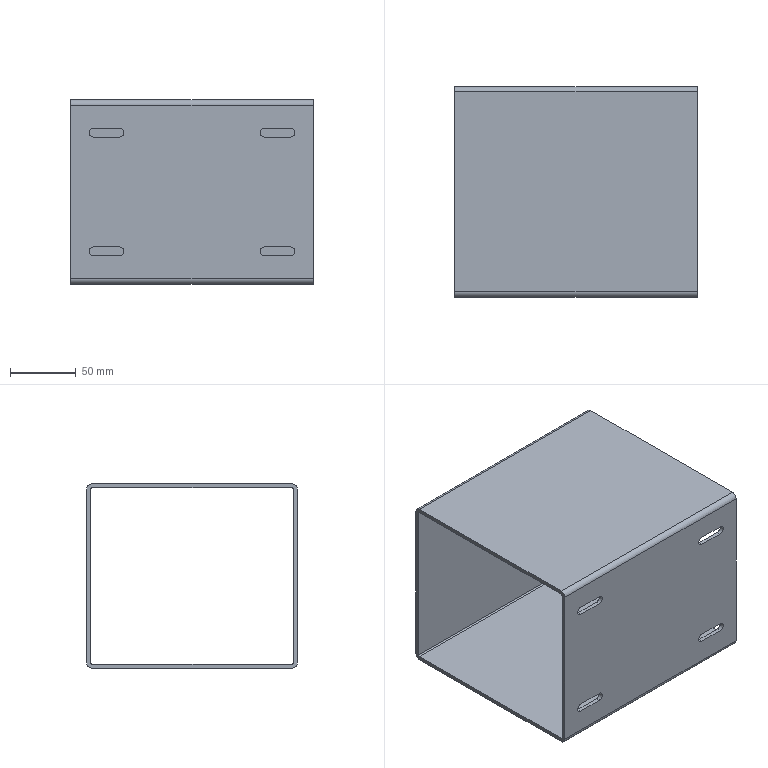Part | SolidWorks | features Fillet 2, Extrusion 1, ICE 1 | 1 solid | 34 faces | box 184 x 160 x 140 mm | volume 320249 mm3 | plane 18 | cylinder 16 | commonest cylinder face diameters 6.5 x8 2 x4 8 x4
STEP:
#1=CARTESIAN_POINT('',(150.,-76.,-70.));
#2=VERTEX_POINT('',#1);
#3=CARTESIAN_POINT('',(150.,76.,-70.));
#4=VERTEX_POINT('',#3);
#5=CARTESIAN_POINT('',(150.,80.,-70.));
#6=DIRECTION('',(0.,1.,0.));
#7=VECTOR('',#6,1000.);
#8=LINE('',#5,#7);
#9=EDGE_CURVE('',#2,#4,#8,.T.);
#10=ORIENTED_EDGE('',*,*,#9,.F.);
#11=CARTESIAN_POINT('',(-34.,-76.,-70.));
#12=VERTEX_POINT('',#11);
#13=CARTESIAN_POINT('',(-34.,-76.,-70.));
#14=DIRECTION('',(-1.,0.,0.));
#15=VECTOR('',#14,1000.);
#16=LINE('',#13,#15);
#17=EDGE_CURVE('',#2,#12,#16,.T.);
#18=ORIENTED_EDGE('',*,*,#17,.T.);
#19=CARTESIAN_POINT('',(-34.,76.,-70.));
#20=VERTEX_POINT('',#19);
#21=CARTESIAN_POINT('',(-34.,80.,-70.));
#22=DIRECTION('',(0.,1.,0.));
#23=VECTOR('',#22,1000.);
#24=LINE('',#21,#23);
#25=EDGE_CURVE('',#12,#20,#24,.T.);
#26=ORIENTED_EDGE('',*,*,#25,.T.);
#27=CARTESIAN_POINT('',(-34.,76.,-70.));
#28=DIRECTION('',(1.,0.,0.));
#29=VECTOR('',#28,1000.);
#30=LINE('',#27,#29);
#31=EDGE_CURVE('',#20,#4,#30,.T.);
#32=ORIENTED_EDGE('',*,*,#31,.T.);
#33=EDGE_LOOP('',(#10,#18,#26,#32));
#34=FACE_OUTER_BOUND('',#33,.T.);
#35=CARTESIAN_POINT('',(-34.,80.,-70.));
#36=DIRECTION('',(0.,0.,-1.));
#37=DIRECTION('',(0.,1.,0.));
#38=AXIS2_PLACEMENT_3D('',#35,#36,#37);
#39=PLANE('',#38);
#40=ADVANCED_FACE('',(#34),#39,.T.);
#41=CARTESIAN_POINT('',(-17.,-80.,48.25));
#42=VERTEX_POINT('',#41);
#43=CARTESIAN_POINT('',(-17.,-80.,41.75));
#44=VERTEX_POINT('',#43);
#45=CARTESIAN_POINT('',(-17.,-80.,45.));
#46=DIRECTION('',(0.,-1.,0.));
#47=DIRECTION('',(0.,0.,-1.));
#48=AXIS2_PLACEMENT_3D('',#45,#46,#47);
#49=CIRCLE('',#48,3.25);
#50=EDGE_CURVE('',#42,#44,#49,.T.);
#51=ORIENTED_EDGE('',*,*,#50,.F.);
#52=CARTESIAN_POINT('',(3.,-80.,48.25));
#53=VERTEX_POINT('',#52);
#54=CARTESIAN_POINT('',(-34.,-80.,48.25));
#55=DIRECTION('',(-1.,0.,0.));
#56=VECTOR('',#55,1000.);
#57=LINE('',#54,#56);
#58=EDGE_CURVE('',#53,#42,#57,.T.);
#59=ORIENTED_EDGE('',*,*,#58,.F.);
#60=CARTESIAN_POINT('',(3.,-80.,41.75));
#61=VERTEX_POINT('',#60);
#62=CARTESIAN_POINT('',(3.,-80.,45.));
#63=DIRECTION('',(0.,-1.,0.));
#64=DIRECTION('',(0.,0.,-1.));
#65=AXIS2_PLACEMENT_3D('',#62,#63,#64);
#66=CIRCLE('',#65,3.25);
#67=EDGE_CURVE('',#61,#53,#66,.T.);
#68=ORIENTED_EDGE('',*,*,#67,.F.);
#69=CARTESIAN_POINT('',(-34.,-80.,41.75));
#70=DIRECTION('',(1.,0.,0.));
#71=VECTOR('',#70,1000.);
#72=LINE('',#69,#71);
#73=EDGE_CURVE('',#44,#61,#72,.T.);
#74=ORIENTED_EDGE('',*,*,#73,.F.);
#75=EDGE_LOOP('',(#51,#59,#68,#74));
#76=FACE_BOUND('',#75,.T.);
#77=CARTESIAN_POINT('',(133.,-80.,-48.25));
#78=VERTEX_POINT('',#77);
#79=CARTESIAN_POINT('',(133.,-80.,-41.75));
#80=VERTEX_POINT('',#79);
#81=CARTESIAN_POINT('',(133.,-80.,-45.));
#82=DIRECTION('',(0.,-1.,0.));
#83=DIRECTION('',(0.,0.,-1.));
#84=AXIS2_PLACEMENT_3D('',#81,#82,#83);
#85=CIRCLE('',#84,3.25);
#86=EDGE_CURVE('',#78,#80,#85,.T.);
#87=ORIENTED_EDGE('',*,*,#86,.F.);
#88=CARTESIAN_POINT('',(113.,-80.,-48.25));
#89=VERTEX_POINT('',#88);
#90=CARTESIAN_POINT('',(-34.,-80.,-48.25));
#91=DIRECTION('',(1.,0.,0.));
#92=VECTOR('',#91,1000.);
#93=LINE('',#90,#92);
#94=EDGE_CURVE('',#89,#78,#93,.T.);
#95=ORIENTED_EDGE('',*,*,#94,.F.);
#96=CARTESIAN_POINT('',(113.,-80.,-41.75));
#97=VERTEX_POINT('',#96);
#98=CARTESIAN_POINT('',(113.,-80.,-45.));
#99=DIRECTION('',(0.,-1.,0.));
#100=DIRECTION('',(0.,0.,-1.));
#101=AXIS2_PLACEMENT_3D('',#98,#99,#100);
#102=CIRCLE('',#101,3.25);
#103=EDGE_CURVE('',#97,#89,#102,.T.);
#104=ORIENTED_EDGE('',*,*,#103,.F.);
#105=CARTESIAN_POINT('',(-34.,-80.,-41.75));
#106=DIRECTION('',(-1.,0.,0.));
#107=VECTOR('',#106,1000.);
#108=LINE('',#105,#107);
#109=EDGE_CURVE('',#80,#97,#108,.T.);
#110=ORIENTED_EDGE('',*,*,#109,.F.);
#111=EDGE_LOOP('',(#87,#95,#104,#110));
#112=FACE_BOUND('',#111,.T.);
#113=CARTESIAN_POINT('',(133.,-80.,41.75));
#114=VERTEX_POINT('',#113);
#115=CARTESIAN_POINT('',(133.,-80.,48.25));
#116=VERTEX_POINT('',#115);
#117=CARTESIAN_POINT('',(133.,-80.,45.));
#118=DIRECTION('',(0.,-1.,0.));
#119=DIRECTION('',(0.,0.,-1.));
#120=AXIS2_PLACEMENT_3D('',#117,#118,#119);
#121=CIRCLE('',#120,3.25);
#122=EDGE_CURVE('',#114,#116,#121,.T.);
#123=ORIENTED_EDGE('',*,*,#122,.F.);
#124=CARTESIAN_POINT('',(113.,-80.,41.75));
#125=VERTEX_POINT('',#124);
#126=CARTESIAN_POINT('',(-34.,-80.,41.75));
#127=DIRECTION('',(1.,0.,0.));
#128=VECTOR('',#127,1000.);
#129=LINE('',#126,#128);
#130=EDGE_CURVE('',#125,#114,#129,.T.);
#131=ORIENTED_EDGE('',*,*,#130,.F.);
#132=CARTESIAN_POINT('',(113.,-80.,48.25));
#133=VERTEX_POINT('',#132);
#134=CARTESIAN_POINT('',(113.,-80.,45.));
#135=DIRECTION('',(0.,-1.,0.));
#136=DIRECTION('',(0.,0.,-1.));
#137=AXIS2_PLACEMENT_3D('',#134,#135,#136);
#138=CIRCLE('',#137,3.25);
#139=EDGE_CURVE('',#133,#125,#138,.T.);
#140=ORIENTED_EDGE('',*,*,#139,.F.);
#141=CARTESIAN_POINT('',(-34.,-80.,48.25));
#142=DIRECTION('',(-1.,0.,0.));
#143=VECTOR('',#142,1000.);
#144=LINE('',#141,#143);
#145=EDGE_CURVE('',#116,#133,#144,.T.);
#146=ORIENTED_EDGE('',*,*,#145,.F.);
#147=EDGE_LOOP('',(#123,#131,#140,#146));
#148=FACE_BOUND('',#147,.T.);
#149=CARTESIAN_POINT('',(-17.,-80.,-41.75));
#150=VERTEX_POINT('',#149);
#151=CARTESIAN_POINT('',(-17.,-80.,-48.25));
#152=VERTEX_POINT('',#151);
#153=CARTESIAN_POINT('',(-17.,-80.,-45.));
#154=DIRECTION('',(0.,-1.,0.));
#155=DIRECTION('',(0.,0.,-1.));
#156=AXIS2_PLACEMENT_3D('',#153,#154,#155);
#157=CIRCLE('',#156,3.25);
#158=EDGE_CURVE('',#150,#152,#157,.T.);
#159=ORIENTED_EDGE('',*,*,#158,.F.);
#160=CARTESIAN_POINT('',(3.,-80.,-41.75));
#161=VERTEX_POINT('',#160);
#162=CARTESIAN_POINT('',(-34.,-80.,-41.75));
#163=DIRECTION('',(-1.,0.,0.));
#164=VECTOR('',#163,1000.);
#165=LINE('',#162,#164);
#166=EDGE_CURVE('',#161,#150,#165,.T.);
#167=ORIENTED_EDGE('',*,*,#166,.F.);
#168=CARTESIAN_POINT('',(3.,-80.,-48.25));
#169=VERTEX_POINT('',#168);
#170=CARTESIAN_POINT('',(3.,-80.,-45.));
#171=DIRECTION('',(0.,-1.,0.));
#172=DIRECTION('',(0.,0.,-1.));
#173=AXIS2_PLACEMENT_3D('',#170,#171,#172);
#174=CIRCLE('',#173,3.25);
#175=EDGE_CURVE('',#169,#161,#174,.T.);
#176=ORIENTED_EDGE('',*,*,#175,.F.);
#177=CARTESIAN_POINT('',(-34.,-80.,-48.25));
#178=DIRECTION('',(1.,0.,0.));
#179=VECTOR('',#178,1000.);
#180=LINE('',#177,#179);
#181=EDGE_CURVE('',#152,#169,#180,.T.);
#182=ORIENTED_EDGE('',*,*,#181,.F.);
#183=EDGE_LOOP('',(#159,#167,#176,#182));
#184=FACE_BOUND('',#183,.T.);
#185=CARTESIAN_POINT('',(150.,-80.,66.));
#186=VERTEX_POINT('',#185);
#187=CARTESIAN_POINT('',(150.,-80.,-66.));
#188=VERTEX_POINT('',#187);
#189=CARTESIAN_POINT('',(150.,-80.,70.));
#190=DIRECTION('',(0.,0.,-1.));
#191=VECTOR('',#190,1000.);
#192=LINE('',#189,#191);
#193=EDGE_CURVE('',#186,#188,#192,.T.);
#194=ORIENTED_EDGE('',*,*,#193,.F.);
#195=CARTESIAN_POINT('',(-34.,-80.,66.));
#196=VERTEX_POINT('',#195);
#197=CARTESIAN_POINT('',(-34.,-80.,66.));
#198=DIRECTION('',(-1.,0.,0.));
#199=VECTOR('',#198,1000.);
#200=LINE('',#197,#199);
#201=EDGE_CURVE('',#186,#196,#200,.T.);
#202=ORIENTED_EDGE('',*,*,#201,.T.);
#203=CARTESIAN_POINT('',(-34.,-80.,-66.));
#204=VERTEX_POINT('',#203);
#205=CARTESIAN_POINT('',(-34.,-80.,70.));
#206=DIRECTION('',(0.,0.,-1.));
#207=VECTOR('',#206,1000.);
#208=LINE('',#205,#207);
#209=EDGE_CURVE('',#196,#204,#208,.T.);
#210=ORIENTED_EDGE('',*,*,#209,.T.);
#211=CARTESIAN_POINT('',(-34.,-80.,-66.));
#212=DIRECTION('',(1.,0.,0.));
#213=VECTOR('',#212,1000.);
#214=LINE('',#211,#213);
#215=EDGE_CURVE('',#204,#188,#214,.T.);
#216=ORIENTED_EDGE('',*,*,#215,.T.);
#217=EDGE_LOOP('',(#194,#202,#210,#216));
#218=FACE_OUTER_BOUND('',#217,.T.);
#219=CARTESIAN_POINT('',(-34.,-80.,70.));
#220=DIRECTION('',(0.,-1.,0.));
#221=DIRECTION('',(0.,0.,-1.));
#222=AXIS2_PLACEMENT_3D('',#219,#220,#221);
#223=PLANE('',#222);
#224=ADVANCED_FACE('',(#76,#112,#148,#184,#218),#223,.T.);
#225=CARTESIAN_POINT('',(-34.,76.,70.));
#226=VERTEX_POINT('',#225);
#227=CARTESIAN_POINT('',(-34.,-76.,70.));
#228=VERTEX_POINT('',#227);
#229=CARTESIAN_POINT('',(-34.,80.,70.));
#230=DIRECTION('',(0.,-1.,0.));
#231=VECTOR('',#230,1000.);
#232=LINE('',#229,#231);
#233=EDGE_CURVE('',#226,#228,#232,.T.);
#234=ORIENTED_EDGE('',*,*,#233,.T.);
#235=CARTESIAN_POINT('',(150.,-76.,70.));
#236=VERTEX_POINT('',#235);
#237=CARTESIAN_POINT('',(-34.,-76.,70.));
#238=DIRECTION('',(1.,0.,0.));
#239=VECTOR('',#238,1000.);
#240=LINE('',#237,#239);
#241=EDGE_CURVE('',#228,#236,#240,.T.);
#242=ORIENTED_EDGE('',*,*,#241,.T.);
#243=CARTESIAN_POINT('',(150.,76.,70.));
#244=VERTEX_POINT('',#243);
#245=CARTESIAN_POINT('',(150.,80.,70.));
#246=DIRECTION('',(0.,-1.,0.));
#247=VECTOR('',#246,1000.);
#248=LINE('',#245,#247);
#249=EDGE_CURVE('',#244,#236,#248,.T.);
#250=ORIENTED_EDGE('',*,*,#249,.F.);
#251=CARTESIAN_POINT('',(-34.,76.,70.));
#252=DIRECTION('',(-1.,0.,0.));
#253=VECTOR('',#252,1000.);
#254=LINE('',#251,#253);
#255=EDGE_CURVE('',#244,#226,#254,.T.);
#256=ORIENTED_EDGE('',*,*,#255,.T.);
#257=EDGE_LOOP('',(#234,#242,#250,#256));
#258=FACE_OUTER_BOUND('',#257,.T.);
#259=CARTESIAN_POINT('',(-34.,80.,70.));
#260=DIRECTION('',(0.,0.,1.));
#261=DIRECTION('',(0.,-1.,0.));
#262=AXIS2_PLACEMENT_3D('',#259,#260,#261);
#263=PLANE('',#262);
#264=ADVANCED_FACE('',(#258),#263,.T.);
#265=CARTESIAN_POINT('',(150.,80.,-66.));
#266=VERTEX_POINT('',#265);
#267=CARTESIAN_POINT('',(150.,80.,66.));
#268=VERTEX_POINT('',#267);
#269=CARTESIAN_POINT('',(150.,80.,70.));
#270=DIRECTION('',(0.,0.,1.));
#271=VECTOR('',#270,1000.);
#272=LINE('',#269,#271);
#273=EDGE_CURVE('',#266,#268,#272,.T.);
#274=ORIENTED_EDGE('',*,*,#273,.F.);
#275=CARTESIAN_POINT('',(-34.,80.,-66.));
#276=VERTEX_POINT('',#275);
#277=CARTESIAN_POINT('',(-34.,80.,-66.));
#278=DIRECTION('',(-1.,0.,0.));
#279=VECTOR('',#278,1000.);
#280=LINE('',#277,#279);
#281=EDGE_CURVE('',#266,#276,#280,.T.);
#282=ORIENTED_EDGE('',*,*,#281,.T.);
#283=CARTESIAN_POINT('',(-34.,80.,66.));
#284=VERTEX_POINT('',#283);
#285=CARTESIAN_POINT('',(-34.,80.,70.));
#286=DIRECTION('',(0.,0.,1.));
#287=VECTOR('',#286,1000.);
#288=LINE('',#285,#287);
#289=EDGE_CURVE('',#276,#284,#288,.T.);
#290=ORIENTED_EDGE('',*,*,#289,.T.);
#291=CARTESIAN_POINT('',(-34.,80.,66.));
#292=DIRECTION('',(1.,0.,0.));
#293=VECTOR('',#292,1000.);
#294=LINE('',#291,#293);
#295=EDGE_CURVE('',#284,#268,#294,.T.);
#296=ORIENTED_EDGE('',*,*,#295,.T.);
#297=EDGE_LOOP('',(#274,#282,#290,#296));
#298=FACE_OUTER_BOUND('',#297,.T.);
#299=CARTESIAN_POINT('',(-34.,80.,70.));
#300=DIRECTION('',(0.,1.,0.));
#301=DIRECTION('',(0.,0.,1.));
#302=AXIS2_PLACEMENT_3D('',#299,#300,#301);
#303=PLANE('',#302);
#304=ADVANCED_FACE('',(#298),#303,.T.);
#305=CARTESIAN_POINT('',(-34.,-76.,-67.));
#306=VERTEX_POINT('',#305);
#307=CARTESIAN_POINT('',(-34.,76.,-67.));
#308=VERTEX_POINT('',#307);
#309=CARTESIAN_POINT('',(-34.,77.,-67.));
#310=DIRECTION('',(0.,1.,0.));
#311=VECTOR('',#310,1000.);
#312=LINE('',#309,#311);
#313=EDGE_CURVE('',#306,#308,#312,.T.);
#314=ORIENTED_EDGE('',*,*,#313,.T.);
#315=CARTESIAN_POINT('',(-34.,77.,-66.));
#316=VERTEX_POINT('',#315);
#317=CARTESIAN_POINT('',(-34.,76.,-66.));
#318=DIRECTION('',(1.,0.,0.));
#319=DIRECTION('',(0.,0.,-1.));
#320=AXIS2_PLACEMENT_3D('',#317,#318,#319);
#321=CIRCLE('',#320,1.);
#322=EDGE_CURVE('',#308,#316,#321,.T.);
#323=ORIENTED_EDGE('',*,*,#322,.T.);
#324=CARTESIAN_POINT('',(-34.,77.,66.));
#325=VERTEX_POINT('',#324);
#326=CARTESIAN_POINT('',(-34.,77.,67.));
#327=DIRECTION('',(0.,0.,1.));
#328=VECTOR('',#327,1000.);
#329=LINE('',#326,#328);
#330=EDGE_CURVE('',#316,#325,#329,.T.);
#331=ORIENTED_EDGE('',*,*,#330,.T.);
#332=CARTESIAN_POINT('',(-34.,76.,67.));
#333=VERTEX_POINT('',#332);
#334=CARTESIAN_POINT('',(-34.,76.,66.));
#335=DIRECTION('',(1.,0.,0.));
#336=DIRECTION('',(0.,0.,-1.));
#337=AXIS2_PLACEMENT_3D('',#334,#335,#336);
#338=CIRCLE('',#337,1.);
#339=EDGE_CURVE('',#325,#333,#338,.T.);
#340=ORIENTED_EDGE('',*,*,#339,.T.);
#341=CARTESIAN_POINT('',(-34.,-76.,67.));
#342=VERTEX_POINT('',#341);
#343=CARTESIAN_POINT('',(-34.,77.,67.));
#344=DIRECTION('',(0.,-1.,0.));
#345=VECTOR('',#344,1000.);
#346=LINE('',#343,#345);
#347=EDGE_CURVE('',#333,#342,#346,.T.);
#348=ORIENTED_EDGE('',*,*,#347,.T.);
#349=CARTESIAN_POINT('',(-34.,-77.,66.));
#350=VERTEX_POINT('',#349);
#351=CARTESIAN_POINT('',(-34.,-76.,66.));
#352=DIRECTION('',(1.,0.,0.));
#353=DIRECTION('',(0.,0.,-1.));
#354=AXIS2_PLACEMENT_3D('',#351,#352,#353);
#355=CIRCLE('',#354,1.);
#356=EDGE_CURVE('',#342,#350,#355,.T.);
#357=ORIENTED_EDGE('',*,*,#356,.T.);
#358=CARTESIAN_POINT('',(-34.,-77.,-66.));
#359=VERTEX_POINT('',#358);
#360=CARTESIAN_POINT('',(-34.,-77.,67.));
#361=DIRECTION('',(0.,0.,-1.));
#362=VECTOR('',#361,1000.);
#363=LINE('',#360,#362);
#364=EDGE_CURVE('',#350,#359,#363,.T.);
#365=ORIENTED_EDGE('',*,*,#364,.T.);
#366=CARTESIAN_POINT('',(-34.,-76.,-66.));
#367=DIRECTION('',(1.,0.,0.));
#368=DIRECTION('',(0.,0.,-1.));
#369=AXIS2_PLACEMENT_3D('',#366,#367,#368);
#370=CIRCLE('',#369,1.);
#371=EDGE_CURVE('',#359,#306,#370,.T.);
#372=ORIENTED_EDGE('',*,*,#371,.T.);
#373=EDGE_LOOP('',(#314,#323,#331,#340,#348,#357,#365,#372));
#374=FACE_BOUND('',#373,.T.);
#375=ORIENTED_EDGE('',*,*,#209,.F.);
#376=CARTESIAN_POINT('',(-34.,-76.,66.));
#377=DIRECTION('',(-1.,0.,0.));
#378=DIRECTION('',(0.,0.,-1.));
#379=AXIS2_PLACEMENT_3D('',#376,#377,#378);
#380=CIRCLE('',#379,4.);
#381=EDGE_CURVE('',#196,#228,#380,.T.);
#382=ORIENTED_EDGE('',*,*,#381,.T.);
#383=ORIENTED_EDGE('',*,*,#233,.F.);
#384=CARTESIAN_POINT('',(-34.,76.,66.));
#385=DIRECTION('',(-1.,0.,0.));
#386=DIRECTION('',(0.,0.,-1.));
#387=AXIS2_PLACEMENT_3D('',#384,#385,#386);
#388=CIRCLE('',#387,4.);
#389=EDGE_CURVE('',#226,#284,#388,.T.);
#390=ORIENTED_EDGE('',*,*,#389,.T.);
#391=ORIENTED_EDGE('',*,*,#289,.F.);
#392=CARTESIAN_POINT('',(-34.,76.,-66.));
#393=DIRECTION('',(-1.,0.,0.));
#394=DIRECTION('',(0.,0.,-1.));
#395=AXIS2_PLACEMENT_3D('',#392,#393,#394);
#396=CIRCLE('',#395,4.);
#397=EDGE_CURVE('',#276,#20,#396,.T.);
#398=ORIENTED_EDGE('',*,*,#397,.T.);
#399=ORIENTED_EDGE('',*,*,#25,.F.);
#400=CARTESIAN_POINT('',(-34.,-76.,-66.));
#401=DIRECTION('',(-1.,0.,0.));
#402=DIRECTION('',(0.,0.,-1.));
#403=AXIS2_PLACEMENT_3D('',#400,#401,#402);
#404=CIRCLE('',#403,4.);
#405=EDGE_CURVE('',#12,#204,#404,.T.);
#406=ORIENTED_EDGE('',*,*,#405,.T.);
#407=EDGE_LOOP('',(#375,#382,#383,#390,#391,#398,#399,#406));
#408=FACE_OUTER_BOUND('',#407,.T.);
#409=CARTESIAN_POINT('',(-34.,0.,0.));
#410=DIRECTION('',(1.,0.,0.));
#411=DIRECTION('',(0.,0.,-1.));
#412=AXIS2_PLACEMENT_3D('',#409,#410,#411);
#413=PLANE('',#412);
#414=ADVANCED_FACE('',(#374,#408),#413,.F.);
#415=ORIENTED_EDGE('',*,*,#347,.F.);
#416=CARTESIAN_POINT('',(150.,76.,67.));
#417=VERTEX_POINT('',#416);
#418=CARTESIAN_POINT('',(150.,76.,67.));
#419=DIRECTION('',(1.,0.,0.));
#420=VECTOR('',#419,1000.);
#421=LINE('',#418,#420);
#422=EDGE_CURVE('',#333,#417,#421,.T.);
#423=ORIENTED_EDGE('',*,*,#422,.T.);
#424=CARTESIAN_POINT('',(150.,-76.,67.));
#425=VERTEX_POINT('',#424);
#426=CARTESIAN_POINT('',(150.,77.,67.));
#427=DIRECTION('',(0.,-1.,0.));
#428=VECTOR('',#427,1000.);
#429=LINE('',#426,#428);
#430=EDGE_CURVE('',#417,#425,#429,.T.);
#431=ORIENTED_EDGE('',*,*,#430,.T.);
#432=CARTESIAN_POINT('',(-34.,-76.,67.));
#433=DIRECTION('',(-1.,0.,0.));
#434=VECTOR('',#433,1000.);
#435=LINE('',#432,#434);
#436=EDGE_CURVE('',#425,#342,#435,.T.);
#437=ORIENTED_EDGE('',*,*,#436,.T.);
#438=EDGE_LOOP('',(#415,#423,#431,#437));
#439=FACE_OUTER_BOUND('',#438,.T.);
#440=CARTESIAN_POINT('',(-34.,77.,67.));
#441=DIRECTION('',(0.,0.,1.));
#442=DIRECTION('',(0.,-1.,0.));
#443=AXIS2_PLACEMENT_3D('',#440,#441,#442);
#444=PLANE('',#443);
#445=ADVANCED_FACE('',(#439),#444,.F.);
#446=ORIENTED_EDGE('',*,*,#330,.F.);
#447=CARTESIAN_POINT('',(150.,77.,-66.));
#448=VERTEX_POINT('',#447);
#449=CARTESIAN_POINT('',(150.,77.,-66.));
#450=DIRECTION('',(1.,0.,0.));
#451=VECTOR('',#450,1000.);
#452=LINE('',#449,#451);
#453=EDGE_CURVE('',#316,#448,#452,.T.);
#454=ORIENTED_EDGE('',*,*,#453,.T.);
#455=CARTESIAN_POINT('',(150.,77.,66.));
#456=VERTEX_POINT('',#455);
#457=CARTESIAN_POINT('',(150.,77.,67.));
#458=DIRECTION('',(0.,0.,1.));
#459=VECTOR('',#458,1000.);
#460=LINE('',#457,#459);
#461=EDGE_CURVE('',#448,#456,#460,.T.);
#462=ORIENTED_EDGE('',*,*,#461,.T.);
#463=CARTESIAN_POINT('',(-34.,77.,66.));
#464=DIRECTION('',(-1.,0.,0.));
#465=VECTOR('',#464,1000.);
#466=LINE('',#463,#465);
#467=EDGE_CURVE('',#456,#325,#466,.T.);
#468=ORIENTED_EDGE('',*,*,#467,.T.);
#469=EDGE_LOOP('',(#446,#454,#462,#468));
#470=FACE_OUTER_BOUND('',#469,.T.);
#471=CARTESIAN_POINT('',(-34.,77.,67.));
#472=DIRECTION('',(0.,1.,0.));
#473=DIRECTION('',(0.,0.,1.));
#474=AXIS2_PLACEMENT_3D('',#471,#472,#473);
#475=PLANE('',#474);
#476=ADVANCED_FACE('',(#470),#475,.F.);
#477=CARTESIAN_POINT('',(150.,-76.,-67.));
#478=VERTEX_POINT('',#477);
#479=CARTESIAN_POINT('',(150.,76.,-67.));
#480=VERTEX_POINT('',#479);
#481=CARTESIAN_POINT('',(150.,77.,-67.));
#482=DIRECTION('',(0.,1.,0.));
#483=VECTOR('',#482,1000.);
#484=LINE('',#481,#483);
#485=EDGE_CURVE('',#478,#480,#484,.T.);
#486=ORIENTED_EDGE('',*,*,#485,.T.);
#487=CARTESIAN_POINT('',(-34.,76.,-67.));
#488=DIRECTION('',(-1.,0.,0.));
#489=VECTOR('',#488,1000.);
#490=LINE('',#487,#489);
#491=EDGE_CURVE('',#480,#308,#490,.T.);
#492=ORIENTED_EDGE('',*,*,#491,.T.);
#493=ORIENTED_EDGE('',*,*,#313,.F.);
#494=CARTESIAN_POINT('',(150.,-76.,-67.));
#495=DIRECTION('',(1.,0.,0.));
#496=VECTOR('',#495,1000.);
#497=LINE('',#494,#496);
#498=EDGE_CURVE('',#306,#478,#497,.T.);
#499=ORIENTED_EDGE('',*,*,#498,.T.);
#500=EDGE_LOOP('',(#486,#492,#493,#499));
#501=FACE_OUTER_BOUND('',#500,.T.);
#502=CARTESIAN_POINT('',(-34.,77.,-67.));
#503=DIRECTION('',(0.,0.,-1.));
#504=DIRECTION('',(0.,1.,0.));
#505=AXIS2_PLACEMENT_3D('',#502,#503,#504);
#506=PLANE('',#505);
#507=ADVANCED_FACE('',(#501),#506,.F.);
#508=CARTESIAN_POINT('',(-17.,-77.,48.25));
#509=VERTEX_POINT('',#508);
#510=CARTESIAN_POINT('',(3.,-77.,48.25));
#511=VERTEX_POINT('',#510);
#512=CARTESIAN_POINT('',(-17.,-77.,48.25));
#513=DIRECTION('',(1.,0.,0.));
#514=VECTOR('',#513,1000.);
#515=LINE('',#512,#514);
#516=EDGE_CURVE('',#509,#511,#515,.T.);
#517=ORIENTED_EDGE('',*,*,#516,.F.);
#518=CARTESIAN_POINT('',(-17.,-77.,41.75));
#519=VERTEX_POINT('',#518);
#520=CARTESIAN_POINT('',(-17.,-77.,45.));
#521=DIRECTION('',(0.,1.,0.));
#522=DIRECTION('',(0.,0.,-1.));
#523=AXIS2_PLACEMENT_3D('',#520,#521,#522);
#524=CIRCLE('',#523,3.25);
#525=EDGE_CURVE('',#519,#509,#524,.T.);
#526=ORIENTED_EDGE('',*,*,#525,.F.);
#527=CARTESIAN_POINT('',(3.,-77.,41.75));
#528=VERTEX_POINT('',#527);
#529=CARTESIAN_POINT('',(-17.,-77.,41.75));
#530=DIRECTION('',(-1.,0.,0.));
#531=VECTOR('',#530,1000.);
#532=LINE('',#529,#531);
#533=EDGE_CURVE('',#528,#519,#532,.T.);
#534=ORIENTED_EDGE('',*,*,#533,.F.);
#535=CARTESIAN_POINT('',(3.,-77.,45.));
#536=DIRECTION('',(0.,1.,0.));
#537=DIRECTION('',(0.,0.,-1.));
#538=AXIS2_PLACEMENT_3D('',#535,#536,#537);
#539=CIRCLE('',#538,3.25);
#540=EDGE_CURVE('',#511,#528,#539,.T.);
#541=ORIENTED_EDGE('',*,*,#540,.F.);
#542=EDGE_LOOP('',(#517,#526,#534,#541));
#543=FACE_BOUND('',#542,.T.);
#544=CARTESIAN_POINT('',(133.,-77.,-48.25));
#545=VERTEX_POINT('',#544);
#546=CARTESIAN_POINT('',(113.,-77.,-48.25));
#547=VERTEX_POINT('',#546);
#548=CARTESIAN_POINT('',(133.,-77.,-48.25));
#549=DIRECTION('',(-1.,0.,0.));
#550=VECTOR('',#549,1000.);
#551=LINE('',#548,#550);
#552=EDGE_CURVE('',#545,#547,#551,.T.);
#553=ORIENTED_EDGE('',*,*,#552,.F.);
#554=CARTESIAN_POINT('',(133.,-77.,-41.75));
#555=VERTEX_POINT('',#554);
#556=CARTESIAN_POINT('',(133.,-77.,-45.));
#557=DIRECTION('',(0.,1.,0.));
#558=DIRECTION('',(0.,0.,-1.));
#559=AXIS2_PLACEMENT_3D('',#556,#557,#558);
#560=CIRCLE('',#559,3.25);
#561=EDGE_CURVE('',#555,#545,#560,.T.);
#562=ORIENTED_EDGE('',*,*,#561,.F.);
#563=CARTESIAN_POINT('',(113.,-77.,-41.75));
#564=VERTEX_POINT('',#563);
#565=CARTESIAN_POINT('',(133.,-77.,-41.75));
#566=DIRECTION('',(1.,0.,0.));
#567=VECTOR('',#566,1000.);
#568=LINE('',#565,#567);
#569=EDGE_CURVE('',#564,#555,#568,.T.);
#570=ORIENTED_EDGE('',*,*,#569,.F.);
#571=CARTESIAN_POINT('',(113.,-77.,-45.));
#572=DIRECTION('',(0.,1.,0.));
#573=DIRECTION('',(0.,0.,-1.));
#574=AXIS2_PLACEMENT_3D('',#571,#572,#573);
#575=CIRCLE('',#574,3.25);
#576=EDGE_CURVE('',#547,#564,#575,.T.);
#577=ORIENTED_EDGE('',*,*,#576,.F.);
#578=EDGE_LOOP('',(#553,#562,#570,#577));
#579=FACE_BOUND('',#578,.T.);
#580=CARTESIAN_POINT('',(133.,-77.,41.75));
#581=VERTEX_POINT('',#580);
#582=CARTESIAN_POINT('',(113.,-77.,41.75));
#583=VERTEX_POINT('',#582);
#584=CARTESIAN_POINT('',(133.,-77.,41.75));
#585=DIRECTION('',(-1.,0.,0.));
#586=VECTOR('',#585,1000.);
#587=LINE('',#584,#586);
#588=EDGE_CURVE('',#581,#583,#587,.T.);
#589=ORIENTED_EDGE('',*,*,#588,.F.);
#590=CARTESIAN_POINT('',(133.,-77.,48.25));
#591=VERTEX_POINT('',#590);
#592=CARTESIAN_POINT('',(133.,-77.,45.));
#593=DIRECTION('',(0.,1.,0.));
#594=DIRECTION('',(0.,0.,1.));
#595=AXIS2_PLACEMENT_3D('',#592,#593,#594);
#596=CIRCLE('',#595,3.25);
#597=EDGE_CURVE('',#591,#581,#596,.T.);
#598=ORIENTED_EDGE('',*,*,#597,.F.);
#599=CARTESIAN_POINT('',(113.,-77.,48.25));
#600=VERTEX_POINT('',#599);
#601=CARTESIAN_POINT('',(133.,-77.,48.25));
#602=DIRECTION('',(1.,0.,0.));
#603=VECTOR('',#602,1000.);
#604=LINE('',#601,#603);
#605=EDGE_CURVE('',#600,#591,#604,.T.);
#606=ORIENTED_EDGE('',*,*,#605,.F.);
#607=CARTESIAN_POINT('',(113.,-77.,45.));
#608=DIRECTION('',(0.,1.,0.));
#609=DIRECTION('',(0.,0.,1.));
#610=AXIS2_PLACEMENT_3D('',#607,#608,#609);
#611=CIRCLE('',#610,3.25);
#612=EDGE_CURVE('',#583,#600,#611,.T.);
#613=ORIENTED_EDGE('',*,*,#612,.F.);
#614=EDGE_LOOP('',(#589,#598,#606,#613));
#615=FACE_BOUND('',#614,.T.);
#616=CARTESIAN_POINT('',(-17.,-77.,-41.75));
#617=VERTEX_POINT('',#616);
#618=CARTESIAN_POINT('',(3.,-77.,-41.75));
#619=VERTEX_POINT('',#618);
#620=CARTESIAN_POINT('',(-17.,-77.,-41.75));
#621=DIRECTION('',(1.,0.,0.));
#622=VECTOR('',#621,1000.);
#623=LINE('',#620,#622);
#624=EDGE_CURVE('',#617,#619,#623,.T.);
#625=ORIENTED_EDGE('',*,*,#624,.F.);
#626=CARTESIAN_POINT('',(-17.,-77.,-48.25));
#627=VERTEX_POINT('',#626);
#628=CARTESIAN_POINT('',(-17.,-77.,-45.));
#629=DIRECTION('',(0.,1.,0.));
#630=DIRECTION('',(0.,0.,1.));
#631=AXIS2_PLACEMENT_3D('',#628,#629,#630);
#632=CIRCLE('',#631,3.25);
#633=EDGE_CURVE('',#627,#617,#632,.T.);
#634=ORIENTED_EDGE('',*,*,#633,.F.);
#635=CARTESIAN_POINT('',(3.,-77.,-48.25));
#636=VERTEX_POINT('',#635);
#637=CARTESIAN_POINT('',(-17.,-77.,-48.25));
#638=DIRECTION('',(-1.,0.,0.));
#639=VECTOR('',#638,1000.);
#640=LINE('',#637,#639);
#641=EDGE_CURVE('',#636,#627,#640,.T.);
#642=ORIENTED_EDGE('',*,*,#641,.F.);
#643=CARTESIAN_POINT('',(3.,-77.,-45.));
#644=DIRECTION('',(0.,1.,0.));
#645=DIRECTION('',(0.,0.,1.));
#646=AXIS2_PLACEMENT_3D('',#643,#644,#645);
#647=CIRCLE('',#646,3.25);
#648=EDGE_CURVE('',#619,#636,#647,.T.);
#649=ORIENTED_EDGE('',*,*,#648,.F.);
#650=EDGE_LOOP('',(#625,#634,#642,#649));
#651=FACE_BOUND('',#650,.T.);
#652=ORIENTED_EDGE('',*,*,#364,.F.);
#653=CARTESIAN_POINT('',(150.,-77.,66.));
#654=VERTEX_POINT('',#653);
#655=CARTESIAN_POINT('',(150.,-77.,66.));
#656=DIRECTION('',(1.,0.,0.));
#657=VECTOR('',#656,1000.);
#658=LINE('',#655,#657);
#659=EDGE_CURVE('',#350,#654,#658,.T.);
#660=ORIENTED_EDGE('',*,*,#659,.T.);
#661=CARTESIAN_POINT('',(150.,-77.,-66.));
#662=VERTEX_POINT('',#661);
#663=CARTESIAN_POINT('',(150.,-77.,67.));
#664=DIRECTION('',(0.,0.,-1.));
#665=VECTOR('',#664,1000.);
#666=LINE('',#663,#665);
#667=EDGE_CURVE('',#654,#662,#666,.T.);
#668=ORIENTED_EDGE('',*,*,#667,.T.);
#669=CARTESIAN_POINT('',(-34.,-77.,-66.));
#670=DIRECTION('',(-1.,0.,0.));
#671=VECTOR('',#670,1000.);
#672=LINE('',#669,#671);
#673=EDGE_CURVE('',#662,#359,#672,.T.);
#674=ORIENTED_EDGE('',*,*,#673,.T.);
#675=EDGE_LOOP('',(#652,#660,#668,#674));
#676=FACE_OUTER_BOUND('',#675,.T.);
#677=CARTESIAN_POINT('',(-34.,-77.,67.));
#678=DIRECTION('',(0.,-1.,0.));
#679=DIRECTION('',(0.,0.,-1.));
#680=AXIS2_PLACEMENT_3D('',#677,#678,#679);
#681=PLANE('',#680);
#682=ADVANCED_FACE('',(#543,#579,#615,#651,#676),#681,.F.);
#683=ORIENTED_EDGE('',*,*,#249,.T.);
#684=CARTESIAN_POINT('',(150.,-76.,66.));
#685=DIRECTION('',(1.,0.,0.));
#686=DIRECTION('',(0.,0.,-1.));
#687=AXIS2_PLACEMENT_3D('',#684,#685,#686);
#688=CIRCLE('',#687,4.);
#689=EDGE_CURVE('',#236,#186,#688,.T.);
#690=ORIENTED_EDGE('',*,*,#689,.T.);
#691=ORIENTED_EDGE('',*,*,#193,.T.);
#692=CARTESIAN_POINT('',(150.,-76.,-66.));
#693=DIRECTION('',(1.,0.,0.));
#694=DIRECTION('',(0.,0.,-1.));
#695=AXIS2_PLACEMENT_3D('',#692,#693,#694);
#696=CIRCLE('',#695,4.);
#697=EDGE_CURVE('',#188,#2,#696,.T.);
#698=ORIENTED_EDGE('',*,*,#697,.T.);
#699=ORIENTED_EDGE('',*,*,#9,.T.);
#700=CARTESIAN_POINT('',(150.,76.,-66.));
#701=DIRECTION('',(1.,0.,0.));
#702=DIRECTION('',(0.,0.,-1.));
#703=AXIS2_PLACEMENT_3D('',#700,#701,#702);
#704=CIRCLE('',#703,4.);
#705=EDGE_CURVE('',#4,#266,#704,.T.);
#706=ORIENTED_EDGE('',*,*,#705,.T.);
#707=ORIENTED_EDGE('',*,*,#273,.T.);
#708=CARTESIAN_POINT('',(150.,76.,66.));
#709=DIRECTION('',(1.,0.,0.));
#710=DIRECTION('',(0.,0.,-1.));
#711=AXIS2_PLACEMENT_3D('',#708,#709,#710);
#712=CIRCLE('',#711,4.);
#713=EDGE_CURVE('',#268,#244,#712,.T.);
#714=ORIENTED_EDGE('',*,*,#713,.T.);
#715=EDGE_LOOP('',(#683,#690,#691,#698,#699,#706,#707,#714));
#716=FACE_OUTER_BOUND('',#715,.T.);
#717=ORIENTED_EDGE('',*,*,#667,.F.);
#718=CARTESIAN_POINT('',(150.,-76.,66.));
#719=DIRECTION('',(-1.,0.,0.));
#720=DIRECTION('',(0.,0.,-1.));
#721=AXIS2_PLACEMENT_3D('',#718,#719,#720);
#722=CIRCLE('',#721,1.);
#723=EDGE_CURVE('',#654,#425,#722,.T.);
#724=ORIENTED_EDGE('',*,*,#723,.T.);
#725=ORIENTED_EDGE('',*,*,#430,.F.);
#726=CARTESIAN_POINT('',(150.,76.,66.));
#727=DIRECTION('',(-1.,0.,0.));
#728=DIRECTION('',(0.,0.,-1.));
#729=AXIS2_PLACEMENT_3D('',#726,#727,#728);
#730=CIRCLE('',#729,1.);
#731=EDGE_CURVE('',#417,#456,#730,.T.);
#732=ORIENTED_EDGE('',*,*,#731,.T.);
#733=ORIENTED_EDGE('',*,*,#461,.F.);
#734=CARTESIAN_POINT('',(150.,76.,-66.));
#735=DIRECTION('',(-1.,0.,0.));
#736=DIRECTION('',(0.,0.,-1.));
#737=AXIS2_PLACEMENT_3D('',#734,#735,#736);
#738=CIRCLE('',#737,1.);
#739=EDGE_CURVE('',#448,#480,#738,.T.);
#740=ORIENTED_EDGE('',*,*,#739,.T.);
#741=ORIENTED_EDGE('',*,*,#485,.F.);
#742=CARTESIAN_POINT('',(150.,-76.,-66.));
#743=DIRECTION('',(-1.,0.,0.));
#744=DIRECTION('',(0.,0.,-1.));
#745=AXIS2_PLACEMENT_3D('',#742,#743,#744);
#746=CIRCLE('',#745,1.);
#747=EDGE_CURVE('',#478,#662,#746,.T.);
#748=ORIENTED_EDGE('',*,*,#747,.T.);
#749=EDGE_LOOP('',(#717,#724,#725,#732,#733,#740,#741,#748));
#750=FACE_BOUND('',#749,.T.);
#751=CARTESIAN_POINT('',(150.,0.,0.));
#752=DIRECTION('',(1.,0.,0.));
#753=DIRECTION('',(0.,0.,-1.));
#754=AXIS2_PLACEMENT_3D('',#751,#752,#753);
#755=PLANE('',#754);
#756=ADVANCED_FACE('',(#716,#750),#755,.T.);
#757=ORIENTED_EDGE('',*,*,#158,.T.);
#758=CARTESIAN_POINT('',(-17.,-87.,-48.25));
#759=DIRECTION('',(0.,1.,0.));
#760=VECTOR('',#759,1000.);
#761=LINE('',#758,#760);
#762=EDGE_CURVE('',#152,#627,#761,.T.);
#763=ORIENTED_EDGE('',*,*,#762,.T.);
#764=ORIENTED_EDGE('',*,*,#633,.T.);
#765=CARTESIAN_POINT('',(-17.,-87.,-41.75));
#766=DIRECTION('',(0.,1.,0.));
#767=VECTOR('',#766,1000.);
#768=LINE('',#765,#767);
#769=EDGE_CURVE('',#150,#617,#768,.T.);
#770=ORIENTED_EDGE('',*,*,#769,.F.);
#771=EDGE_LOOP('',(#757,#763,#764,#770));
#772=FACE_OUTER_BOUND('',#771,.T.);
#773=CARTESIAN_POINT('',(-17.,-87.,-45.));
#774=DIRECTION('',(0.,1.,0.));
#775=DIRECTION('',(0.,0.,1.));
#776=AXIS2_PLACEMENT_3D('',#773,#774,#775);
#777=CYLINDRICAL_SURFACE('',#776,3.25);
#778=ADVANCED_FACE('',(#772),#777,.F.);
#779=ORIENTED_EDGE('',*,*,#181,.T.);
#780=CARTESIAN_POINT('',(3.,-87.,-48.25));
#781=DIRECTION('',(0.,1.,0.));
#782=VECTOR('',#781,1000.);
#783=LINE('',#780,#782);
#784=EDGE_CURVE('',#169,#636,#783,.T.);
#785=ORIENTED_EDGE('',*,*,#784,.T.);
#786=ORIENTED_EDGE('',*,*,#641,.T.);
#787=ORIENTED_EDGE('',*,*,#762,.F.);
#788=EDGE_LOOP('',(#779,#785,#786,#787));
#789=FACE_OUTER_BOUND('',#788,.T.);
#790=CARTESIAN_POINT('',(-17.,-87.,-48.25));
#791=DIRECTION('',(0.,0.,-1.));
#792=DIRECTION('',(-1.,0.,0.));
#793=AXIS2_PLACEMENT_3D('',#790,#791,#792);
#794=PLANE('',#793);
#795=ADVANCED_FACE('',(#789),#794,.F.);
#796=ORIENTED_EDGE('',*,*,#175,.T.);
#797=CARTESIAN_POINT('',(3.,-87.,-41.75));
#798=DIRECTION('',(0.,1.,0.));
#799=VECTOR('',#798,1000.);
#800=LINE('',#797,#799);
#801=EDGE_CURVE('',#161,#619,#800,.T.);
#802=ORIENTED_EDGE('',*,*,#801,.T.);
#803=ORIENTED_EDGE('',*,*,#648,.T.);
#804=ORIENTED_EDGE('',*,*,#784,.F.);
#805=EDGE_LOOP('',(#796,#802,#803,#804));
#806=FACE_OUTER_BOUND('',#805,.T.);
#807=CARTESIAN_POINT('',(3.,-87.,-45.));
#808=DIRECTION('',(0.,1.,0.));
#809=DIRECTION('',(0.,0.,1.));
#810=AXIS2_PLACEMENT_3D('',#807,#808,#809);
#811=CYLINDRICAL_SURFACE('',#810,3.25);
#812=ADVANCED_FACE('',(#806),#811,.F.);
#813=ORIENTED_EDGE('',*,*,#166,.T.);
#814=ORIENTED_EDGE('',*,*,#769,.T.);
#815=ORIENTED_EDGE('',*,*,#624,.T.);
#816=ORIENTED_EDGE('',*,*,#801,.F.);
#817=EDGE_LOOP('',(#813,#814,#815,#816));
#818=FACE_OUTER_BOUND('',#817,.T.);
#819=CARTESIAN_POINT('',(-17.,-87.,-41.75));
#820=DIRECTION('',(0.,0.,1.));
#821=DIRECTION('',(1.,0.,0.));
#822=AXIS2_PLACEMENT_3D('',#819,#820,#821);
#823=PLANE('',#822);
#824=ADVANCED_FACE('',(#818),#823,.F.);
#825=ORIENTED_EDGE('',*,*,#122,.T.);
#826=CARTESIAN_POINT('',(133.,-87.,48.25));
#827=DIRECTION('',(0.,1.,0.));
#828=VECTOR('',#827,1000.);
#829=LINE('',#826,#828);
#830=EDGE_CURVE('',#116,#591,#829,.T.);
#831=ORIENTED_EDGE('',*,*,#830,.T.);
#832=ORIENTED_EDGE('',*,*,#597,.T.);
#833=CARTESIAN_POINT('',(133.,-87.,41.75));
#834=DIRECTION('',(0.,1.,0.));
#835=VECTOR('',#834,1000.);
#836=LINE('',#833,#835);
#837=EDGE_CURVE('',#114,#581,#836,.T.);
#838=ORIENTED_EDGE('',*,*,#837,.F.);
#839=EDGE_LOOP('',(#825,#831,#832,#838));
#840=FACE_OUTER_BOUND('',#839,.T.);
#841=CARTESIAN_POINT('',(133.,-87.,45.));
#842=DIRECTION('',(0.,1.,0.));
#843=DIRECTION('',(0.,0.,1.));
#844=AXIS2_PLACEMENT_3D('',#841,#842,#843);
#845=CYLINDRICAL_SURFACE('',#844,3.25);
#846=ADVANCED_FACE('',(#840),#845,.F.);
#847=ORIENTED_EDGE('',*,*,#145,.T.);
#848=CARTESIAN_POINT('',(113.,-87.,48.25));
#849=DIRECTION('',(0.,1.,0.));
#850=VECTOR('',#849,1000.);
#851=LINE('',#848,#850);
#852=EDGE_CURVE('',#133,#600,#851,.T.);
#853=ORIENTED_EDGE('',*,*,#852,.T.);
#854=ORIENTED_EDGE('',*,*,#605,.T.);
#855=ORIENTED_EDGE('',*,*,#830,.F.);
#856=EDGE_LOOP('',(#847,#853,#854,#855));
#857=FACE_OUTER_BOUND('',#856,.T.);
#858=CARTESIAN_POINT('',(133.,-87.,48.25));
#859=DIRECTION('',(0.,0.,1.));
#860=DIRECTION('',(1.,0.,0.));
#861=AXIS2_PLACEMENT_3D('',#858,#859,#860);
#862=PLANE('',#861);
#863=ADVANCED_FACE('',(#857),#862,.F.);
#864=ORIENTED_EDGE('',*,*,#139,.T.);
#865=CARTESIAN_POINT('',(113.,-87.,41.75));
#866=DIRECTION('',(0.,1.,0.));
#867=VECTOR('',#866,1000.);
#868=LINE('',#865,#867);
#869=EDGE_CURVE('',#125,#583,#868,.T.);
#870=ORIENTED_EDGE('',*,*,#869,.T.);
#871=ORIENTED_EDGE('',*,*,#612,.T.);
#872=ORIENTED_EDGE('',*,*,#852,.F.);
#873=EDGE_LOOP('',(#864,#870,#871,#872));
#874=FACE_OUTER_BOUND('',#873,.T.);
#875=CARTESIAN_POINT('',(113.,-87.,45.));
#876=DIRECTION('',(0.,1.,0.));
#877=DIRECTION('',(0.,0.,1.));
#878=AXIS2_PLACEMENT_3D('',#875,#876,#877);
#879=CYLINDRICAL_SURFACE('',#878,3.25);
#880=ADVANCED_FACE('',(#874),#879,.F.);
#881=ORIENTED_EDGE('',*,*,#130,.T.);
#882=ORIENTED_EDGE('',*,*,#837,.T.);
#883=ORIENTED_EDGE('',*,*,#588,.T.);
#884=ORIENTED_EDGE('',*,*,#869,.F.);
#885=EDGE_LOOP('',(#881,#882,#883,#884));
#886=FACE_OUTER_BOUND('',#885,.T.);
#887=CARTESIAN_POINT('',(133.,-87.,41.75));
#888=DIRECTION('',(0.,0.,-1.));
#889=DIRECTION('',(-1.,0.,0.));
#890=AXIS2_PLACEMENT_3D('',#887,#888,#889);
#891=PLANE('',#890);
#892=ADVANCED_FACE('',(#886),#891,.F.);
#893=ORIENTED_EDGE('',*,*,#86,.T.);
#894=CARTESIAN_POINT('',(133.,-87.,-41.75));
#895=DIRECTION('',(0.,1.,0.));
#896=VECTOR('',#895,1000.);
#897=LINE('',#894,#896);
#898=EDGE_CURVE('',#80,#555,#897,.T.);
#899=ORIENTED_EDGE('',*,*,#898,.T.);
#900=ORIENTED_EDGE('',*,*,#561,.T.);
#901=CARTESIAN_POINT('',(133.,-87.,-48.25));
#902=DIRECTION('',(0.,1.,0.));
#903=VECTOR('',#902,1000.);
#904=LINE('',#901,#903);
#905=EDGE_CURVE('',#78,#545,#904,.T.);
#906=ORIENTED_EDGE('',*,*,#905,.F.);
#907=EDGE_LOOP('',(#893,#899,#900,#906));
#908=FACE_OUTER_BOUND('',#907,.T.);
#909=CARTESIAN_POINT('',(133.,-87.,-45.));
#910=DIRECTION('',(0.,1.,0.));
#911=DIRECTION('',(0.,0.,1.));
#912=AXIS2_PLACEMENT_3D('',#909,#910,#911);
#913=CYLINDRICAL_SURFACE('',#912,3.25);
#914=ADVANCED_FACE('',(#908),#913,.F.);
#915=ORIENTED_EDGE('',*,*,#109,.T.);
#916=CARTESIAN_POINT('',(113.,-87.,-41.75));
#917=DIRECTION('',(0.,1.,0.));
#918=VECTOR('',#917,1000.);
#919=LINE('',#916,#918);
#920=EDGE_CURVE('',#97,#564,#919,.T.);
#921=ORIENTED_EDGE('',*,*,#920,.T.);
#922=ORIENTED_EDGE('',*,*,#569,.T.);
#923=ORIENTED_EDGE('',*,*,#898,.F.);
#924=EDGE_LOOP('',(#915,#921,#922,#923));
#925=FACE_OUTER_BOUND('',#924,.T.);
#926=CARTESIAN_POINT('',(133.,-87.,-41.75));
#927=DIRECTION('',(0.,0.,1.));
#928=DIRECTION('',(1.,0.,0.));
#929=AXIS2_PLACEMENT_3D('',#926,#927,#928);
#930=PLANE('',#929);
#931=ADVANCED_FACE('',(#925),#930,.F.);
#932=ORIENTED_EDGE('',*,*,#103,.T.);
#933=CARTESIAN_POINT('',(113.,-87.,-48.25));
#934=DIRECTION('',(0.,1.,0.));
#935=VECTOR('',#934,1000.);
#936=LINE('',#933,#935);
#937=EDGE_CURVE('',#89,#547,#936,.T.);
#938=ORIENTED_EDGE('',*,*,#937,.T.);
#939=ORIENTED_EDGE('',*,*,#576,.T.);
#940=ORIENTED_EDGE('',*,*,#920,.F.);
#941=EDGE_LOOP('',(#932,#938,#939,#940));
#942=FACE_OUTER_BOUND('',#941,.T.);
#943=CARTESIAN_POINT('',(113.,-87.,-45.));
#944=DIRECTION('',(0.,1.,0.));
#945=DIRECTION('',(0.,0.,1.));
#946=AXIS2_PLACEMENT_3D('',#943,#944,#945);
#947=CYLINDRICAL_SURFACE('',#946,3.25);
#948=ADVANCED_FACE('',(#942),#947,.F.);
#949=ORIENTED_EDGE('',*,*,#94,.T.);
#950=ORIENTED_EDGE('',*,*,#905,.T.);
#951=ORIENTED_EDGE('',*,*,#552,.T.);
#952=ORIENTED_EDGE('',*,*,#937,.F.);
#953=EDGE_LOOP('',(#949,#950,#951,#952));
#954=FACE_OUTER_BOUND('',#953,.T.);
#955=CARTESIAN_POINT('',(133.,-87.,-48.25));
#956=DIRECTION('',(0.,0.,-1.));
#957=DIRECTION('',(-1.,0.,0.));
#958=AXIS2_PLACEMENT_3D('',#955,#956,#957);
#959=PLANE('',#958);
#960=ADVANCED_FACE('',(#954),#959,.F.);
#961=ORIENTED_EDGE('',*,*,#50,.T.);
#962=CARTESIAN_POINT('',(-17.,-87.,41.75));
#963=DIRECTION('',(0.,1.,0.));
#964=VECTOR('',#963,1000.);
#965=LINE('',#962,#964);
#966=EDGE_CURVE('',#44,#519,#965,.T.);
#967=ORIENTED_EDGE('',*,*,#966,.T.);
#968=ORIENTED_EDGE('',*,*,#525,.T.);
#969=CARTESIAN_POINT('',(-17.,-87.,48.25));
#970=DIRECTION('',(0.,1.,0.));
#971=VECTOR('',#970,1000.);
#972=LINE('',#969,#971);
#973=EDGE_CURVE('',#42,#509,#972,.T.);
#974=ORIENTED_EDGE('',*,*,#973,.F.);
#975=EDGE_LOOP('',(#961,#967,#968,#974));
#976=FACE_OUTER_BOUND('',#975,.T.);
#977=CARTESIAN_POINT('',(-17.,-87.,45.));
#978=DIRECTION('',(0.,1.,0.));
#979=DIRECTION('',(0.,0.,1.));
#980=AXIS2_PLACEMENT_3D('',#977,#978,#979);
#981=CYLINDRICAL_SURFACE('',#980,3.25);
#982=ADVANCED_FACE('',(#976),#981,.F.);
#983=ORIENTED_EDGE('',*,*,#73,.T.);
#984=CARTESIAN_POINT('',(3.,-87.,41.75));
#985=DIRECTION('',(0.,1.,0.));
#986=VECTOR('',#985,1000.);
#987=LINE('',#984,#986);
#988=EDGE_CURVE('',#61,#528,#987,.T.);
#989=ORIENTED_EDGE('',*,*,#988,.T.);
#990=ORIENTED_EDGE('',*,*,#533,.T.);
#991=ORIENTED_EDGE('',*,*,#966,.F.);
#992=EDGE_LOOP('',(#983,#989,#990,#991));
#993=FACE_OUTER_BOUND('',#992,.T.);
#994=CARTESIAN_POINT('',(-17.,-87.,41.75));
#995=DIRECTION('',(0.,0.,-1.));
#996=DIRECTION('',(-1.,0.,0.));
#997=AXIS2_PLACEMENT_3D('',#994,#995,#996);
#998=PLANE('',#997);
#999=ADVANCED_FACE('',(#993),#998,.F.);
#1000=ORIENTED_EDGE('',*,*,#67,.T.);
#1001=CARTESIAN_POINT('',(3.,-87.,48.25));
#1002=DIRECTION('',(0.,1.,0.));
#1003=VECTOR('',#1002,1000.);
#1004=LINE('',#1001,#1003);
#1005=EDGE_CURVE('',#53,#511,#1004,.T.);
#1006=ORIENTED_EDGE('',*,*,#1005,.T.);
#1007=ORIENTED_EDGE('',*,*,#540,.T.);
#1008=ORIENTED_EDGE('',*,*,#988,.F.);
#1009=EDGE_LOOP('',(#1000,#1006,#1007,#1008));
#1010=FACE_OUTER_BOUND('',#1009,.T.);
#1011=CARTESIAN_POINT('',(3.,-87.,45.));
#1012=DIRECTION('',(0.,1.,0.));
#1013=DIRECTION('',(0.,0.,1.));
#1014=AXIS2_PLACEMENT_3D('',#1011,#1012,#1013);
#1015=CYLINDRICAL_SURFACE('',#1014,3.25);
#1016=ADVANCED_FACE('',(#1010),#1015,.F.);
#1017=ORIENTED_EDGE('',*,*,#58,.T.);
#1018=ORIENTED_EDGE('',*,*,#973,.T.);
#1019=ORIENTED_EDGE('',*,*,#516,.T.);
#1020=ORIENTED_EDGE('',*,*,#1005,.F.);
#1021=EDGE_LOOP('',(#1017,#1018,#1019,#1020));
#1022=FACE_OUTER_BOUND('',#1021,.T.);
#1023=CARTESIAN_POINT('',(-17.,-87.,48.25));
#1024=DIRECTION('',(0.,0.,1.));
#1025=DIRECTION('',(1.,0.,0.));
#1026=AXIS2_PLACEMENT_3D('',#1023,#1024,#1025);
#1027=PLANE('',#1026);
#1028=ADVANCED_FACE('',(#1022),#1027,.F.);
#1029=ORIENTED_EDGE('',*,*,#322,.F.);
#1030=ORIENTED_EDGE('',*,*,#491,.F.);
#1031=ORIENTED_EDGE('',*,*,#739,.F.);
#1032=ORIENTED_EDGE('',*,*,#453,.F.);
#1033=EDGE_LOOP('',(#1029,#1030,#1031,#1032));
#1034=FACE_OUTER_BOUND('',#1033,.T.);
#1035=CARTESIAN_POINT('',(-34.,76.,-66.));
#1036=DIRECTION('',(-1.,0.,0.));
#1037=DIRECTION('',(0.,0.,1.));
#1038=AXIS2_PLACEMENT_3D('',#1035,#1036,#1037);
#1039=CYLINDRICAL_SURFACE('',#1038,1.);
#1040=ADVANCED_FACE('',(#1034),#1039,.F.);
#1041=ORIENTED_EDGE('',*,*,#339,.F.);
#1042=ORIENTED_EDGE('',*,*,#467,.F.);
#1043=ORIENTED_EDGE('',*,*,#731,.F.);
#1044=ORIENTED_EDGE('',*,*,#422,.F.);
#1045=EDGE_LOOP('',(#1041,#1042,#1043,#1044));
#1046=FACE_OUTER_BOUND('',#1045,.T.);
#1047=CARTESIAN_POINT('',(-34.,76.,66.));
#1048=DIRECTION('',(-1.,0.,0.));
#1049=DIRECTION('',(0.,0.,1.));
#1050=AXIS2_PLACEMENT_3D('',#1047,#1048,#1049);
#1051=CYLINDRICAL_SURFACE('',#1050,1.);
#1052=ADVANCED_FACE('',(#1046),#1051,.F.);
#1053=ORIENTED_EDGE('',*,*,#356,.F.);
#1054=ORIENTED_EDGE('',*,*,#436,.F.);
#1055=ORIENTED_EDGE('',*,*,#723,.F.);
#1056=ORIENTED_EDGE('',*,*,#659,.F.);
#1057=EDGE_LOOP('',(#1053,#1054,#1055,#1056));
#1058=FACE_OUTER_BOUND('',#1057,.T.);
#1059=CARTESIAN_POINT('',(-34.,-76.,66.));
#1060=DIRECTION('',(-1.,0.,0.));
#1061=DIRECTION('',(0.,0.,1.));
#1062=AXIS2_PLACEMENT_3D('',#1059,#1060,#1061);
#1063=CYLINDRICAL_SURFACE('',#1062,1.);
#1064=ADVANCED_FACE('',(#1058),#1063,.F.);
#1065=ORIENTED_EDGE('',*,*,#371,.F.);
#1066=ORIENTED_EDGE('',*,*,#673,.F.);
#1067=ORIENTED_EDGE('',*,*,#747,.F.);
#1068=ORIENTED_EDGE('',*,*,#498,.F.);
#1069=EDGE_LOOP('',(#1065,#1066,#1067,#1068));
#1070=FACE_OUTER_BOUND('',#1069,.T.);
#1071=CARTESIAN_POINT('',(-34.,-76.,-66.));
#1072=DIRECTION('',(-1.,0.,0.));
#1073=DIRECTION('',(0.,0.,1.));
#1074=AXIS2_PLACEMENT_3D('',#1071,#1072,#1073);
#1075=CYLINDRICAL_SURFACE('',#1074,1.);
#1076=ADVANCED_FACE('',(#1070),#1075,.F.);
#1077=ORIENTED_EDGE('',*,*,#381,.F.);
#1078=ORIENTED_EDGE('',*,*,#201,.F.);
#1079=ORIENTED_EDGE('',*,*,#689,.F.);
#1080=ORIENTED_EDGE('',*,*,#241,.F.);
#1081=EDGE_LOOP('',(#1077,#1078,#1079,#1080));
#1082=FACE_OUTER_BOUND('',#1081,.T.);
#1083=CARTESIAN_POINT('',(-34.,-76.,66.));
#1084=DIRECTION('',(1.,0.,0.));
#1085=DIRECTION('',(0.,0.,-1.));
#1086=AXIS2_PLACEMENT_3D('',#1083,#1084,#1085);
#1087=CYLINDRICAL_SURFACE('',#1086,4.);
#1088=ADVANCED_FACE('',(#1082),#1087,.T.);
#1089=ORIENTED_EDGE('',*,*,#405,.F.);
#1090=ORIENTED_EDGE('',*,*,#17,.F.);
#1091=ORIENTED_EDGE('',*,*,#697,.F.);
#1092=ORIENTED_EDGE('',*,*,#215,.F.);
#1093=EDGE_LOOP('',(#1089,#1090,#1091,#1092));
#1094=FACE_OUTER_BOUND('',#1093,.T.);
#1095=CARTESIAN_POINT('',(-34.,-76.,-66.));
#1096=DIRECTION('',(1.,0.,0.));
#1097=DIRECTION('',(0.,0.,-1.));
#1098=AXIS2_PLACEMENT_3D('',#1095,#1096,#1097);
#1099=CYLINDRICAL_SURFACE('',#1098,4.);
#1100=ADVANCED_FACE('',(#1094),#1099,.T.);
#1101=ORIENTED_EDGE('',*,*,#397,.F.);
#1102=ORIENTED_EDGE('',*,*,#281,.F.);
#1103=ORIENTED_EDGE('',*,*,#705,.F.);
#1104=ORIENTED_EDGE('',*,*,#31,.F.);
#1105=EDGE_LOOP('',(#1101,#1102,#1103,#1104));
#1106=FACE_OUTER_BOUND('',#1105,.T.);
#1107=CARTESIAN_POINT('',(-34.,76.,-66.));
#1108=DIRECTION('',(1.,0.,0.));
#1109=DIRECTION('',(0.,0.,-1.));
#1110=AXIS2_PLACEMENT_3D('',#1107,#1108,#1109);
#1111=CYLINDRICAL_SURFACE('',#1110,4.);
#1112=ADVANCED_FACE('',(#1106),#1111,.T.);
#1113=ORIENTED_EDGE('',*,*,#389,.F.);
#1114=ORIENTED_EDGE('',*,*,#255,.F.);
#1115=ORIENTED_EDGE('',*,*,#713,.F.);
#1116=ORIENTED_EDGE('',*,*,#295,.F.);
#1117=EDGE_LOOP('',(#1113,#1114,#1115,#1116));
#1118=FACE_OUTER_BOUND('',#1117,.T.);
#1119=CARTESIAN_POINT('',(-34.,76.,66.));
#1120=DIRECTION('',(1.,0.,0.));
#1121=DIRECTION('',(0.,0.,-1.));
#1122=AXIS2_PLACEMENT_3D('',#1119,#1120,#1121);
#1123=CYLINDRICAL_SURFACE('',#1122,4.);
#1124=ADVANCED_FACE('',(#1118),#1123,.T.);
#1125=CLOSED_SHELL('',(#40,#224,#264,#304,#414,#445,#476,#507,#682,#756,#778,#795,#812,#824,#846,#863,#880,#892,#914,#931,#948,#960,#982,#999,#1016,#1028,#1040,#1052,#1064,#1076,#1088,#1100,#1112,#1124));
#1126=MANIFOLD_SOLID_BREP('',#1125);
#1127=CARTESIAN_POINT('',(0.,0.,0.));
#1128=DIRECTION('',(0.,0.,1.));
#1129=DIRECTION('',(1.,0.,0.));
#1130=AXIS2_PLACEMENT_3D('',#1127,#1128,#1129);
#1131=(LENGTH_UNIT()NAMED_UNIT(*)SI_UNIT(.MILLI.,.METRE.));
#1132=UNCERTAINTY_MEASURE_WITH_UNIT(LENGTH_MEASURE(0.00001),#1131,'','');
#1133=(NAMED_UNIT(*)PLANE_ANGLE_UNIT()SI_UNIT($,.RADIAN.));
#1134=(NAMED_UNIT(*)SI_UNIT($,.STERADIAN.)SOLID_ANGLE_UNIT());
#1135=(GEOMETRIC_REPRESENTATION_CONTEXT(3)GLOBAL_UNCERTAINTY_ASSIGNED_CONTEXT((#1132))GLOBAL_UNIT_ASSIGNED_CONTEXT((#1131,#1133,#1134))REPRESENTATION_CONTEXT('',''));
#1136=ADVANCED_BREP_SHAPE_REPRESENTATION('',(#1126,#1130),#1135);